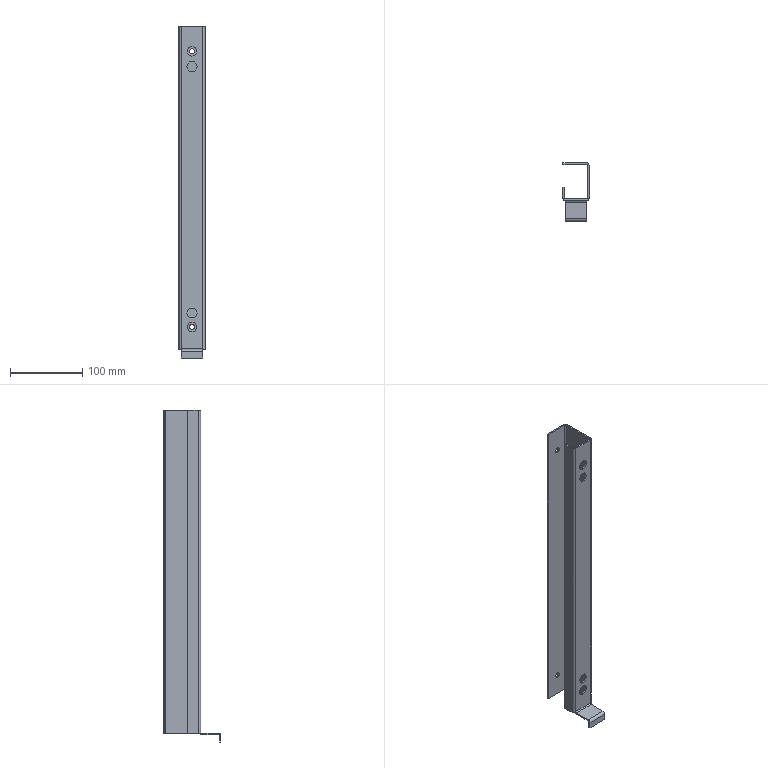Part | STEP file | 1 solid | 68 faces | box 36 x 80 x 458 mm | volume 119357 mm3 | plane 50 | cylinder 18 | commonest cylinder face diameters 7 x9 3 x5 13 x4